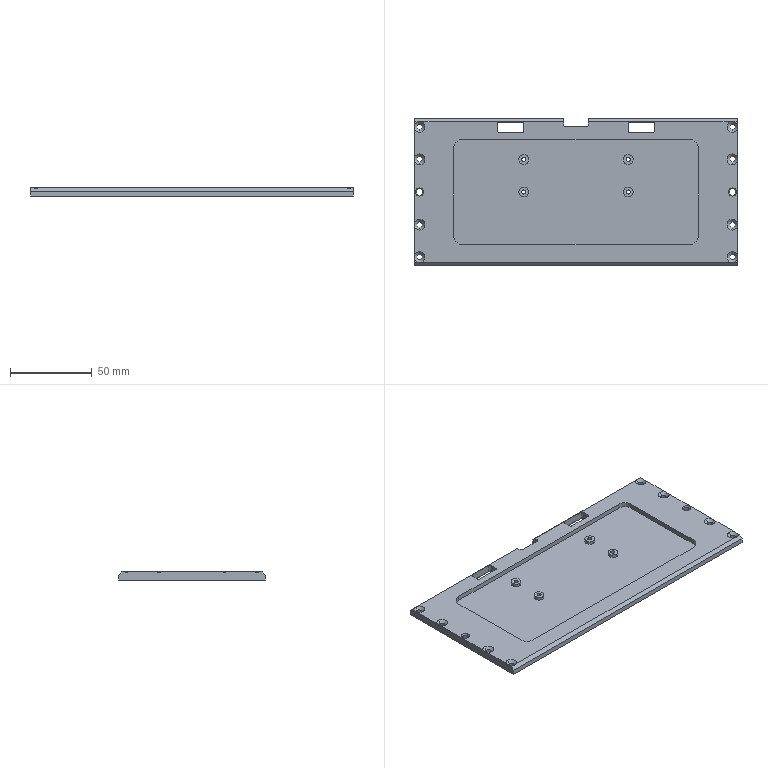NC program | NX | posted with a generic post | part box 198 x 90 x 5 mm
Lines 1 to 1736 of 7766:
N10 G17 G21 G94 G90
(DRILLING , TOOL : D6A45)
N12 T01 M6
N14 G54
N16 G17 G0 G90 X96. Y0. S5000 M3
N18 G43 Z30. H1
N20 G94 G81 G98 Z-2.5 F350. R3.
N22 X-96.
N24 G80
N26 G0 X-96. Y0. Z30.
(DRILLING_COPY_COPY , TOOL : D6A45)
N28 X96. Y-40.
N30 G81 Z-1. F350. R3.
N32 Y-20.
N34 Y20.
N36 Y40.
N38 X32. Y20.
N40 Y0.
N42 X-32.
N44 Y20.
N46 X-96. Y40.
N48 Y20.
N50 Y-20.
N52 Y-40.
N54 G80
N56 G0 X-96. Y-40. Z30.
N58 M5
(DRILLING_COPY_1_COPY , TOOL : 3.4ZT)
N60 T16 M6
N62 G54
N64 G17 G0 G90 X-96. Y-40. S2000 M3
N66 G43 Z30. H16
N68 G94 G83 G98 Z-6.521 F200. Q2. R3.
N70 Y-20.
N72 Y20.
N74 Y40.
N76 X96.
N78 Y20.
N80 Y-20.
N82 Y-40.
N84 G80
N86 G0 X96. Y-40. Z30.
N88 M5
(DRILLING_COPY_1_COPY_COPY , TOOL : 2.5ZT)
N90 T02 M6
N92 G54
N94 G17 G0 G90 X32. Y0. S2000 M3
N96 G43 Z30. H2
N98 G94 G83 G98 Z-6.251 F200. Q2. R3.
N100 Y20.
N102 X-32. Y0.
N104 Y20.
N106 G80
N108 G0 X-32. Y20. Z30.
N110 M5
(ZLEVEL_PROFILE_COPY_1_COPY , TOOL : D10)
N112 T15 M6
N114 G54
N116 G17 G0 G90 X104.1 Y-13.918 S9500 M3
N118 G43 Z30. H15
N120 Z1.5
N122 G94 G1 Y-45.554 Z-0.158 F1000.
N124 X103.766 Y-46.898 Z-0.231
N126 X103.084 Y-48.104 Z-0.303
N128 X102.104 Y-49.084 Z-0.376
N130 X100.898 Y-49.766 Z-0.448
N132 X99.554 Y-50.1 Z-0.521
N134 X99. Z-0.55
N136 X-99. F3000.
N138 G2 X-104.1 Y-45. R5.1
N140 G1 Y45.
N142 G2 X-99. Y50.1 R5.1
N144 G1 X-7.5
N146 G2 X-2.401 Y45.1 R5.1
N148 G1 X2.401
N150 G2 X7.5 Y50.1 R5.1
N152 G1 X99.
N154 G2 X104.1 Y45. R5.1
N156 G1 Y-45.
N158 G2 X99. Y-50.1 R5.1
N160 G1 X-89.1 Z-0.719
N162 X-94.05 Z-0.723
N164 X-99. Z-0.727
N166 X-99.5 Y-50.075 Z-0.728
N168 X-99.995 Y-50.002
N170 X-100.48 Y-49.88 Z-0.729
N172 X-100.952 Y-49.712
N174 X-101.404 Y-49.498 Z-0.73
N176 X-101.833 Y-49.24
N178 X-102.235 Y-48.942 Z-0.731
N180 X-102.606 Y-48.606
N182 X-102.942 Y-48.235 Z-0.732
N184 X-103.24 Y-47.833
N186 X-103.498 Y-47.404
N188 X-103.712 Y-46.952 Z-0.733
N190 X-103.88 Y-46.48
N192 X-104.002 Y-45.995 Z-0.734
N194 X-104.075 Y-45.5
N196 X-104.1 Y-45. Z-0.735
N198 X-104.103 Y-40. Z-0.739
N200 X-104.1 Y-35. Z-0.744
N202 Y35. Z-0.806
N204 X-104.103 Y40. Z-0.811
N206 X-104.1 Y45. Z-0.815
N208 X-104.075 Y45.5 Z-0.816
N210 X-104.002 Y45.995
N212 X-103.88 Y46.48 Z-0.817
N214 X-103.712 Y46.952
N216 X-103.498 Y47.404 Z-0.818
N218 X-103.24 Y47.833
N220 X-102.942 Y48.235
N222 X-102.606 Y48.606 Z-0.819
N224 X-102.235 Y48.942
N226 X-101.833 Y49.24 Z-0.82
N228 X-101.404 Y49.498
N230 X-100.952 Y49.712 Z-0.821
N232 X-100.48 Y49.88
N234 X-99.995 Y50.002 Z-0.822
N236 X-99.5 Y50.075
N238 X-99. Y50.1
N240 X-7.5 Z-0.905
N242 X-7.006 Y50.076
N244 X-6.517 Y50.004
N246 X-6.038 Y49.886 Z-0.906
N248 X-5.571 Y49.721
N250 X-5.123 Y49.512 Z-0.907
N252 X-4.698 Y49.261
N254 X-4.299 Y48.97 Z-0.908
N256 X-3.929 Y48.641
N258 X-3.594 Y48.279
N260 X-3.295 Y47.885 Z-0.909
N262 X-3.035 Y47.465
N264 X-2.817 Y47.021 Z-0.91
N266 X-2.644 Y46.558
N268 X-2.516 Y46.081 Z-0.911
N270 X-2.436 Y45.603
N272 X-2.401 Y45.1 Z-0.912
N274 X2.401 Z-0.916
N276 X2.436 Y45.603
N278 X2.516 Y46.081 Z-0.917
N280 X2.644 Y46.558
N282 X2.817 Y47.021 Z-0.918
N284 X3.035 Y47.465
N286 X3.295 Y47.885 Z-0.919
N288 X3.594 Y48.279
N290 X3.929 Y48.641
N292 X4.299 Y48.97 Z-0.92
N294 X4.698 Y49.261
N296 X5.123 Y49.512 Z-0.921
N298 X5.571 Y49.721
N300 X6.038 Y49.886 Z-0.922
N302 X6.517 Y50.004
N304 X7.006 Y50.076 Z-0.923
N306 X7.5 Y50.1
N308 X99. Z-1.005
N310 X99.5 Y50.075
N312 X99.995 Y50.002 Z-1.006
N314 X100.48 Y49.88
N316 X100.952 Y49.712 Z-1.007
N318 X101.404 Y49.498
N320 X101.833 Y49.24 Z-1.008
N322 X102.235 Y48.942
N324 X102.606 Y48.606 Z-1.009
N326 X102.942 Y48.235
N328 X103.24 Y47.833
N330 X103.498 Y47.404 Z-1.01
N332 X103.712 Y46.952
N334 X103.88 Y46.48 Z-1.011
N336 X104.002 Y45.995
N338 X104.075 Y45.5 Z-1.012
N340 X104.1 Y45.
N342 X104.105 Y40.5 Z-1.016
N344 X104.1 Y36. Z-1.02
N346 Y-36. Z-1.085
N348 X104.105 Y-40.5 Z-1.089
N350 X104.1 Y-45. Z-1.093
N352 X104.075 Y-45.5
N354 X104.002 Y-45.995 Z-1.094
N356 X103.88 Y-46.48
N358 X103.712 Y-46.952 Z-1.095
N360 X103.498 Y-47.404
N362 X103.24 Y-47.833 Z-1.096
N364 X102.942 Y-48.235
N366 X102.606 Y-48.606
N368 X102.235 Y-48.942 Z-1.097
N370 X101.833 Y-49.24
N372 X101.404 Y-49.498 Z-1.098
N374 X100.952 Y-49.712
N376 X100.48 Y-49.88 Z-1.099
N378 X99.995 Y-50.002
N380 X99.5 Y-50.075 Z-1.1
N382 X99. Y-50.1
N384 X-89.1 Z-1.269
N386 X-94.05 Z-1.273
N388 X-99. Z-1.277
N390 X-99.5 Y-50.075 Z-1.278
N392 X-99.995 Y-50.002
N394 X-100.48 Y-49.88 Z-1.279
N396 X-100.952 Y-49.712
N398 X-101.404 Y-49.498 Z-1.28
N400 X-101.833 Y-49.24
N402 X-102.235 Y-48.942 Z-1.281
N404 X-102.606 Y-48.606
N406 X-102.942 Y-48.235 Z-1.282
N408 X-103.24 Y-47.833
N410 X-103.498 Y-47.404
N412 X-103.712 Y-46.952 Z-1.283
N414 X-103.88 Y-46.48
N416 X-104.002 Y-45.995 Z-1.284
N418 X-104.075 Y-45.5
N420 X-104.1 Y-45. Z-1.285
N422 X-104.103 Y-40. Z-1.289
N424 X-104.1 Y-35. Z-1.294
N426 Y35. Z-1.356
N428 X-104.103 Y40. Z-1.361
N430 X-104.1 Y45. Z-1.365
N432 X-104.075 Y45.5 Z-1.366
N434 X-104.002 Y45.995
N436 X-103.88 Y46.48 Z-1.367
N438 X-103.712 Y46.952
N440 X-103.498 Y47.404 Z-1.368
N442 X-103.24 Y47.833
N444 X-102.942 Y48.235
N446 X-102.606 Y48.606 Z-1.369
N448 X-102.235 Y48.942
N450 X-101.833 Y49.24 Z-1.37
N452 X-101.404 Y49.498
N454 X-100.952 Y49.712 Z-1.371
N456 X-100.48 Y49.88
N458 X-99.995 Y50.002 Z-1.372
N460 X-99.5 Y50.075
N462 X-99. Y50.1
N464 X-7.5 Z-1.455
N466 X-7.006 Y50.076
N468 X-6.517 Y50.004
N470 X-6.038 Y49.886 Z-1.456
N472 X-5.571 Y49.721
N474 X-5.123 Y49.512 Z-1.457
N476 X-4.698 Y49.261
N478 X-4.299 Y48.97 Z-1.458
N480 X-3.929 Y48.641
N482 X-3.594 Y48.279
N484 X-3.295 Y47.885 Z-1.459
N486 X-3.035 Y47.465
N488 X-2.817 Y47.021 Z-1.46
N490 X-2.644 Y46.558
N492 X-2.516 Y46.081 Z-1.461
N494 X-2.436 Y45.603
N496 X-2.401 Y45.1 Z-1.462
N498 X2.401 Z-1.466
N500 X2.436 Y45.603
N502 X2.516 Y46.081 Z-1.467
N504 X2.644 Y46.558
N506 X2.817 Y47.021 Z-1.468
N508 X3.035 Y47.465
N510 X3.295 Y47.885 Z-1.469
N512 X3.594 Y48.279
N514 X3.929 Y48.641
N516 X4.299 Y48.97 Z-1.47
N518 X4.698 Y49.261
N520 X5.123 Y49.512 Z-1.471
N522 X5.571 Y49.721
N524 X6.038 Y49.886 Z-1.472
N526 X6.517 Y50.004
N528 X7.006 Y50.076 Z-1.473
N530 X7.5 Y50.1
N532 X99. Z-1.555
N534 X99.5 Y50.075
N536 X99.995 Y50.002 Z-1.556
N538 X100.48 Y49.88
N540 X100.952 Y49.712 Z-1.557
N542 X101.404 Y49.498
N544 X101.833 Y49.24 Z-1.558
N546 X102.235 Y48.942
N548 X102.606 Y48.606 Z-1.559
N550 X102.942 Y48.235
N552 X103.24 Y47.833
N554 X103.498 Y47.404 Z-1.56
N556 X103.712 Y46.952
N558 X103.88 Y46.48 Z-1.561
N560 X104.002 Y45.995
N562 X104.075 Y45.5 Z-1.562
N564 X104.1 Y45.
N566 X104.105 Y40.5 Z-1.566
N568 X104.1 Y36. Z-1.57
N570 Y-36. Z-1.635
N572 X104.105 Y-40.5 Z-1.639
N574 X104.1 Y-45. Z-1.643
N576 X104.075 Y-45.5
N578 X104.002 Y-45.995 Z-1.644
N580 X103.88 Y-46.48
N582 X103.712 Y-46.952 Z-1.645
N584 X103.498 Y-47.404
N586 X103.24 Y-47.833 Z-1.646
N588 X102.942 Y-48.235
N590 X102.606 Y-48.606
N592 X102.235 Y-48.942 Z-1.647
N594 X101.833 Y-49.24
N596 X101.404 Y-49.498 Z-1.648
N598 X100.952 Y-49.712
N600 X100.48 Y-49.88 Z-1.649
N602 X99.995 Y-50.002
N604 X99.5 Y-50.075 Z-1.65
N606 X99. Y-50.1
N608 X-89.1 Z-1.819
N610 X-94.05 Z-1.823
N612 X-99. Z-1.827
N614 X-99.5 Y-50.075 Z-1.828
N616 X-99.995 Y-50.002
N618 X-100.48 Y-49.88 Z-1.829
N620 X-100.952 Y-49.712
N622 X-101.404 Y-49.498 Z-1.83
N624 X-101.833 Y-49.24
N626 X-102.235 Y-48.942 Z-1.831
N628 X-102.606 Y-48.606
N630 X-102.942 Y-48.235 Z-1.832
N632 X-103.24 Y-47.833
N634 X-103.498 Y-47.404
N636 X-103.712 Y-46.952 Z-1.833
N638 X-103.88 Y-46.48
N640 X-104.002 Y-45.995 Z-1.834
N642 X-104.075 Y-45.5
N644 X-104.1 Y-45. Z-1.835
N646 X-104.103 Y-40. Z-1.839
N648 X-104.1 Y-35. Z-1.844
N650 Y35. Z-1.906
N652 X-104.103 Y40. Z-1.911
N654 X-104.1 Y45. Z-1.915
N656 X-104.075 Y45.5 Z-1.916
N658 X-104.002 Y45.995
N660 X-103.88 Y46.48 Z-1.917
N662 X-103.712 Y46.952
N664 X-103.498 Y47.404 Z-1.918
N666 X-103.24 Y47.833
N668 X-102.942 Y48.235
N670 X-102.606 Y48.606 Z-1.919
N672 X-102.235 Y48.942
N674 X-101.833 Y49.24 Z-1.92
N676 X-101.404 Y49.498
N678 X-100.952 Y49.712 Z-1.921
N680 X-100.48 Y49.88
N682 X-99.995 Y50.002 Z-1.922
N684 X-99.5 Y50.075
N686 X-99. Y50.1
N688 X-7.5 Z-2.005
N690 X-7.006 Y50.076
N692 X-6.517 Y50.004
N694 X-6.038 Y49.886 Z-2.006
N696 X-5.571 Y49.721
N698 X-5.123 Y49.512 Z-2.007
N700 X-4.698 Y49.261
N702 X-4.299 Y48.97 Z-2.008
N704 X-3.929 Y48.641
N706 X-3.594 Y48.279
N708 X-3.295 Y47.885 Z-2.009
N710 X-3.035 Y47.465
N712 X-2.817 Y47.021 Z-2.01
N714 X-2.644 Y46.558
N716 X-2.516 Y46.081 Z-2.011
N718 X-2.436 Y45.603
N720 X-2.401 Y45.1 Z-2.012
N722 X2.401 Z-2.016
N724 X2.436 Y45.603
N726 X2.516 Y46.081 Z-2.017
N728 X2.644 Y46.558
N730 X2.817 Y47.021 Z-2.018
N732 X3.035 Y47.465
N734 X3.295 Y47.885 Z-2.019
N736 X3.594 Y48.279
N738 X3.929 Y48.641
N740 X4.299 Y48.97 Z-2.02
N742 X4.698 Y49.261
N744 X5.123 Y49.512 Z-2.021
N746 X5.571 Y49.721
N748 X6.038 Y49.886 Z-2.022
N750 X6.517 Y50.004
N752 X7.006 Y50.076 Z-2.023
N754 X7.5 Y50.1
N756 X99. Z-2.105
N758 X99.5 Y50.075
N760 X99.995 Y50.002 Z-2.106
N762 X100.48 Y49.88
N764 X100.952 Y49.712 Z-2.107
N766 X101.404 Y49.498
N768 X101.833 Y49.24 Z-2.108
N770 X102.235 Y48.942
N772 X102.606 Y48.606 Z-2.109
N774 X102.942 Y48.235
N776 X103.24 Y47.833
N778 X103.498 Y47.404 Z-2.11
N780 X103.712 Y46.952
N782 X103.88 Y46.48 Z-2.111
N784 X104.002 Y45.995
N786 X104.075 Y45.5 Z-2.112
N788 X104.1 Y45.
N790 X104.105 Y40.5 Z-2.116
N792 X104.1 Y36. Z-2.12
N794 Y-36. Z-2.185
N796 X104.105 Y-40.5 Z-2.189
N798 X104.1 Y-45. Z-2.193
N800 X104.075 Y-45.5
N802 X104.002 Y-45.995 Z-2.194
N804 X103.88 Y-46.48
N806 X103.712 Y-46.952 Z-2.195
N808 X103.498 Y-47.404
N810 X103.24 Y-47.833 Z-2.196
N812 X102.942 Y-48.235
N814 X102.606 Y-48.606
N816 X102.235 Y-48.942 Z-2.197
N818 X101.833 Y-49.24
N820 X101.404 Y-49.498 Z-2.198
N822 X100.952 Y-49.712
N824 X100.48 Y-49.88 Z-2.199
N826 X99.995 Y-50.002
N828 X99.5 Y-50.075 Z-2.2
N830 X99. Y-50.1
N832 X-89.1 Z-2.369
N834 X-94.05 Z-2.373
N836 X-99. Z-2.377
N838 X-99.5 Y-50.075 Z-2.378
N840 X-99.995 Y-50.002
N842 X-100.48 Y-49.88 Z-2.379
N844 X-100.952 Y-49.712
N846 X-101.404 Y-49.498 Z-2.38
N848 X-101.833 Y-49.24
N850 X-102.235 Y-48.942 Z-2.381
N852 X-102.606 Y-48.606
N854 X-102.942 Y-48.235 Z-2.382
N856 X-103.24 Y-47.833
N858 X-103.498 Y-47.404
N860 X-103.712 Y-46.952 Z-2.383
N862 X-103.88 Y-46.48
N864 X-104.002 Y-45.995 Z-2.384
N866 X-104.075 Y-45.5
N868 X-104.1 Y-45. Z-2.385
N870 X-104.103 Y-40. Z-2.389
N872 X-104.1 Y-35. Z-2.394
N874 Y35. Z-2.456
N876 X-104.103 Y40. Z-2.461
N878 X-104.1 Y45. Z-2.465
N880 X-104.075 Y45.5 Z-2.466
N882 X-104.002 Y45.995
N884 X-103.88 Y46.48 Z-2.467
N886 X-103.712 Y46.952
N888 X-103.498 Y47.404 Z-2.468
N890 X-103.24 Y47.833
N892 X-102.942 Y48.235
N894 X-102.606 Y48.606 Z-2.469
N896 X-102.235 Y48.942
N898 X-101.833 Y49.24 Z-2.47
N900 X-101.404 Y49.498
N902 X-100.952 Y49.712 Z-2.471
N904 X-100.48 Y49.88
N906 X-99.995 Y50.002 Z-2.472
N908 X-99.5 Y50.075
N910 X-99. Y50.1
N912 X-7.5 Z-2.555
N914 X-7.006 Y50.076
N916 X-6.517 Y50.004
N918 X-6.038 Y49.886 Z-2.556
N920 X-5.571 Y49.721
N922 X-5.123 Y49.512 Z-2.557
N924 X-4.698 Y49.261
N926 X-4.299 Y48.97 Z-2.558
N928 X-3.929 Y48.641
N930 X-3.594 Y48.279
N932 X-3.295 Y47.885 Z-2.559
N934 X-3.035 Y47.465
N936 X-2.817 Y47.021 Z-2.56
N938 X-2.644 Y46.558
N940 X-2.516 Y46.081 Z-2.561
N942 X-2.436 Y45.603
N944 X-2.401 Y45.1 Z-2.562
N946 X2.401 Z-2.566
N948 X2.436 Y45.603
N950 X2.516 Y46.081 Z-2.567
N952 X2.644 Y46.558
N954 X2.817 Y47.021 Z-2.568
N956 X3.035 Y47.465
N958 X3.295 Y47.885 Z-2.569
N960 X3.594 Y48.279
N962 X3.929 Y48.641
N964 X4.299 Y48.97 Z-2.57
N966 X4.698 Y49.261
N968 X5.123 Y49.512 Z-2.571
N970 X5.571 Y49.721
N972 X6.038 Y49.886 Z-2.572
N974 X6.517 Y50.004
N976 X7.006 Y50.076 Z-2.573
N978 X7.5 Y50.1
N980 X99. Z-2.655
N982 X99.5 Y50.075
N984 X99.995 Y50.002 Z-2.656
N986 X100.48 Y49.88
N988 X100.952 Y49.712 Z-2.657
N990 X101.404 Y49.498
N992 X101.833 Y49.24 Z-2.658
N994 X102.235 Y48.942
N996 X102.606 Y48.606 Z-2.659
N998 X102.942 Y48.235
N1000 X103.24 Y47.833
N1002 X103.498 Y47.404 Z-2.66
N1004 X103.712 Y46.952
N1006 X103.88 Y46.48 Z-2.661
N1008 X104.002 Y45.995
N1010 X104.075 Y45.5 Z-2.662
N1012 X104.1 Y45.
N1014 X104.105 Y40.5 Z-2.666
N1016 X104.1 Y36. Z-2.67
N1018 Y-36. Z-2.735
N1020 X104.105 Y-40.5 Z-2.739
N1022 X104.1 Y-45. Z-2.743
N1024 X104.075 Y-45.5
N1026 X104.002 Y-45.995 Z-2.744
N1028 X103.88 Y-46.48
N1030 X103.712 Y-46.952 Z-2.745
N1032 X103.498 Y-47.404
N1034 X103.24 Y-47.833 Z-2.746
N1036 X102.942 Y-48.235
N1038 X102.606 Y-48.606
N1040 X102.235 Y-48.942 Z-2.747
N1042 X101.833 Y-49.24
N1044 X101.404 Y-49.498 Z-2.748
N1046 X100.952 Y-49.712
N1048 X100.48 Y-49.88 Z-2.749
N1050 X99.995 Y-50.002
N1052 X99.5 Y-50.075 Z-2.75
N1054 X99. Y-50.1
N1056 X-89.1 Z-2.919
N1058 X-94.05 Z-2.923
N1060 X-99. Z-2.927
N1062 X-99.5 Y-50.075 Z-2.928
N1064 X-99.995 Y-50.002
N1066 X-100.48 Y-49.88 Z-2.929
N1068 X-100.952 Y-49.712
N1070 X-101.404 Y-49.498 Z-2.93
N1072 X-101.833 Y-49.24
N1074 X-102.235 Y-48.942 Z-2.931
N1076 X-102.606 Y-48.606
N1078 X-102.942 Y-48.235 Z-2.932
N1080 X-103.24 Y-47.833
N1082 X-103.498 Y-47.404
N1084 X-103.712 Y-46.952 Z-2.933
N1086 X-103.88 Y-46.48
N1088 X-104.002 Y-45.995 Z-2.934
N1090 X-104.075 Y-45.5
N1092 X-104.1 Y-45. Z-2.935
N1094 X-104.103 Y-40. Z-2.939
N1096 X-104.1 Y-35. Z-2.944
N1098 Y35. Z-3.006
N1100 X-104.103 Y40. Z-3.011
N1102 X-104.1 Y45. Z-3.015
N1104 X-104.075 Y45.5 Z-3.016
N1106 X-104.002 Y45.995
N1108 X-103.88 Y46.48 Z-3.017
N1110 X-103.712 Y46.952
N1112 X-103.498 Y47.404 Z-3.018
N1114 X-103.24 Y47.833
N1116 X-102.942 Y48.235
N1118 X-102.606 Y48.606 Z-3.019
N1120 X-102.235 Y48.942
N1122 X-101.833 Y49.24 Z-3.02
N1124 X-101.404 Y49.498
N1126 X-100.952 Y49.712 Z-3.021
N1128 X-100.48 Y49.88
N1130 X-99.995 Y50.002 Z-3.022
N1132 X-99.5 Y50.075
N1134 X-99. Y50.1
N1136 X-7.5 Z-3.105
N1138 X-7.006 Y50.076
N1140 X-6.517 Y50.004
N1142 X-6.038 Y49.886 Z-3.106
N1144 X-5.571 Y49.721
N1146 X-5.123 Y49.512 Z-3.107
N1148 X-4.698 Y49.261
N1150 X-4.299 Y48.97 Z-3.108
N1152 X-3.929 Y48.641
N1154 X-3.594 Y48.279
N1156 X-3.295 Y47.885 Z-3.109
N1158 X-3.035 Y47.465
N1160 X-2.817 Y47.021 Z-3.11
N1162 X-2.644 Y46.558
N1164 X-2.516 Y46.081 Z-3.111
N1166 X-2.436 Y45.603
N1168 X-2.401 Y45.1 Z-3.112
N1170 X2.401 Z-3.116
N1172 X2.436 Y45.603
N1174 X2.516 Y46.081 Z-3.117
N1176 X2.644 Y46.558
N1178 X2.817 Y47.021 Z-3.118
N1180 X3.035 Y47.465
N1182 X3.295 Y47.885 Z-3.119
N1184 X3.594 Y48.279
N1186 X3.929 Y48.641
N1188 X4.299 Y48.97 Z-3.12
N1190 X4.698 Y49.261
N1192 X5.123 Y49.512 Z-3.121
N1194 X5.571 Y49.721
N1196 X6.038 Y49.886 Z-3.122
N1198 X6.517 Y50.004
N1200 X7.006 Y50.076 Z-3.123
N1202 X7.5 Y50.1
N1204 X99. Z-3.205
N1206 X99.5 Y50.075
N1208 X99.995 Y50.002 Z-3.206
N1210 X100.48 Y49.88
N1212 X100.952 Y49.712 Z-3.207
N1214 X101.404 Y49.498
N1216 X101.833 Y49.24 Z-3.208
N1218 X102.235 Y48.942
N1220 X102.606 Y48.606 Z-3.209
N1222 X102.942 Y48.235
N1224 X103.24 Y47.833
N1226 X103.498 Y47.404 Z-3.21
N1228 X103.712 Y46.952
N1230 X103.88 Y46.48 Z-3.211
N1232 X104.002 Y45.995
N1234 X104.075 Y45.5 Z-3.212
N1236 X104.1 Y45.
N1238 X104.105 Y40.5 Z-3.216
N1240 X104.1 Y36. Z-3.22
N1242 Y-36. Z-3.285
N1244 X104.105 Y-40.5 Z-3.289
N1246 X104.1 Y-45. Z-3.293
N1248 X104.075 Y-45.5
N1250 X104.002 Y-45.995 Z-3.294
N1252 X103.88 Y-46.48
N1254 X103.712 Y-46.952 Z-3.295
N1256 X103.498 Y-47.404
N1258 X103.24 Y-47.833 Z-3.296
N1260 X102.942 Y-48.235
N1262 X102.606 Y-48.606
N1264 X102.235 Y-48.942 Z-3.297
N1266 X101.833 Y-49.24
N1268 X101.404 Y-49.498 Z-3.298
N1270 X100.952 Y-49.712
N1272 X100.48 Y-49.88 Z-3.299
N1274 X99.995 Y-50.002
N1276 X99.5 Y-50.075 Z-3.3
N1278 X99. Y-50.1
N1280 X-89.1 Z-3.469
N1282 X-94.05 Z-3.473
N1284 X-99. Z-3.477
N1286 X-99.5 Y-50.075 Z-3.478
N1288 X-99.995 Y-50.002
N1290 X-100.48 Y-49.88 Z-3.479
N1292 X-100.952 Y-49.712
N1294 X-101.404 Y-49.498 Z-3.48
N1296 X-101.833 Y-49.24
N1298 X-102.235 Y-48.942 Z-3.481
N1300 X-102.606 Y-48.606
N1302 X-102.942 Y-48.235 Z-3.482
N1304 X-103.24 Y-47.833
N1306 X-103.498 Y-47.404
N1308 X-103.712 Y-46.952 Z-3.483
N1310 X-103.88 Y-46.48
N1312 X-104.002 Y-45.995 Z-3.484
N1314 X-104.075 Y-45.5
N1316 X-104.1 Y-45. Z-3.485
N1318 X-104.103 Y-40. Z-3.489
N1320 X-104.1 Y-35. Z-3.494
N1322 Y35. Z-3.556
N1324 X-104.103 Y40. Z-3.561
N1326 X-104.1 Y45. Z-3.565
N1328 X-104.075 Y45.5 Z-3.566
N1330 X-104.002 Y45.995
N1332 X-103.88 Y46.48 Z-3.567
N1334 X-103.712 Y46.952
N1336 X-103.498 Y47.404 Z-3.568
N1338 X-103.24 Y47.833
N1340 X-102.942 Y48.235
N1342 X-102.606 Y48.606 Z-3.569
N1344 X-102.235 Y48.942
N1346 X-101.833 Y49.24 Z-3.57
N1348 X-101.404 Y49.498
N1350 X-100.952 Y49.712 Z-3.571
N1352 X-100.48 Y49.88
N1354 X-99.995 Y50.002 Z-3.572
N1356 X-99.5 Y50.075
N1358 X-99. Y50.1
N1360 X-7.5 Z-3.655
N1362 X-7.006 Y50.076
N1364 X-6.517 Y50.004
N1366 X-6.038 Y49.886 Z-3.656
N1368 X-5.571 Y49.721
N1370 X-5.123 Y49.512 Z-3.657
N1372 X-4.698 Y49.261
N1374 X-4.299 Y48.97 Z-3.658
N1376 X-3.929 Y48.641
N1378 X-3.594 Y48.279
N1380 X-3.295 Y47.885 Z-3.659
N1382 X-3.035 Y47.465
N1384 X-2.817 Y47.021 Z-3.66
N1386 X-2.644 Y46.558
N1388 X-2.516 Y46.081 Z-3.661
N1390 X-2.436 Y45.603
N1392 X-2.401 Y45.1 Z-3.662
N1394 X2.401 Z-3.666
N1396 X2.436 Y45.603
N1398 X2.516 Y46.081 Z-3.667
N1400 X2.644 Y46.558
N1402 X2.817 Y47.021 Z-3.668
N1404 X3.035 Y47.465
N1406 X3.295 Y47.885 Z-3.669
N1408 X3.594 Y48.279
N1410 X3.929 Y48.641
N1412 X4.299 Y48.97 Z-3.67
N1414 X4.698 Y49.261
N1416 X5.123 Y49.512 Z-3.671
N1418 X5.571 Y49.721
N1420 X6.038 Y49.886 Z-3.672
N1422 X6.517 Y50.004
N1424 X7.006 Y50.076 Z-3.673
N1426 X7.5 Y50.1
N1428 X99. Z-3.755
N1430 X99.5 Y50.075
N1432 X99.995 Y50.002 Z-3.756
N1434 X100.48 Y49.88
N1436 X100.952 Y49.712 Z-3.757
N1438 X101.404 Y49.498
N1440 X101.833 Y49.24 Z-3.758
N1442 X102.235 Y48.942
N1444 X102.606 Y48.606 Z-3.759
N1446 X102.942 Y48.235
N1448 X103.24 Y47.833
N1450 X103.498 Y47.404 Z-3.76
N1452 X103.712 Y46.952
N1454 X103.88 Y46.48 Z-3.761
N1456 X104.002 Y45.995
N1458 X104.075 Y45.5 Z-3.762
N1460 X104.1 Y45.
N1462 X104.105 Y40.5 Z-3.766
N1464 X104.1 Y36. Z-3.77
N1466 Y-36. Z-3.835
N1468 X104.105 Y-40.5 Z-3.839
N1470 X104.1 Y-45. Z-3.843
N1472 X104.075 Y-45.5
N1474 X104.002 Y-45.995 Z-3.844
N1476 X103.88 Y-46.48
N1478 X103.712 Y-46.952 Z-3.845
N1480 X103.498 Y-47.404
N1482 X103.24 Y-47.833 Z-3.846
N1484 X102.942 Y-48.235
N1486 X102.606 Y-48.606
N1488 X102.235 Y-48.942 Z-3.847
N1490 X101.833 Y-49.24
N1492 X101.404 Y-49.498 Z-3.848
N1494 X100.952 Y-49.712
N1496 X100.48 Y-49.88 Z-3.849
N1498 X99.995 Y-50.002
N1500 X99.5 Y-50.075 Z-3.85
N1502 X99. Y-50.1
N1504 X-89.1 Z-4.019
N1506 X-94.05 Z-4.023
N1508 X-99. Z-4.027
N1510 X-99.5 Y-50.075 Z-4.028
N1512 X-99.995 Y-50.002
N1514 X-100.48 Y-49.88 Z-4.029
N1516 X-100.952 Y-49.712
N1518 X-101.404 Y-49.498 Z-4.03
N1520 X-101.833 Y-49.24
N1522 X-102.235 Y-48.942 Z-4.031
N1524 X-102.606 Y-48.606
N1526 X-102.942 Y-48.235 Z-4.032
N1528 X-103.24 Y-47.833
N1530 X-103.498 Y-47.404
N1532 X-103.712 Y-46.952 Z-4.033
N1534 X-103.88 Y-46.48
N1536 X-104.002 Y-45.995 Z-4.034
N1538 X-104.075 Y-45.5
N1540 X-104.1 Y-45. Z-4.035
N1542 X-104.103 Y-40. Z-4.039
N1544 X-104.1 Y-35. Z-4.044
N1546 Y35. Z-4.106
N1548 X-104.103 Y40. Z-4.111
N1550 X-104.1 Y45. Z-4.115
N1552 X-104.075 Y45.5 Z-4.116
N1554 X-104.002 Y45.995
N1556 X-103.88 Y46.48 Z-4.117
N1558 X-103.712 Y46.952
N1560 X-103.498 Y47.404 Z-4.118
N1562 X-103.24 Y47.833
N1564 X-102.942 Y48.235
N1566 X-102.606 Y48.606 Z-4.119
N1568 X-102.235 Y48.942
N1570 X-101.833 Y49.24 Z-4.12
N1572 X-101.404 Y49.498
N1574 X-100.952 Y49.712 Z-4.121
N1576 X-100.48 Y49.88
N1578 X-99.995 Y50.002 Z-4.122
N1580 X-99.5 Y50.075
N1582 X-99. Y50.1
N1584 X-7.5 Z-4.205
N1586 X-7.006 Y50.076
N1588 X-6.517 Y50.004
N1590 X-6.038 Y49.886 Z-4.206
N1592 X-5.571 Y49.721
N1594 X-5.123 Y49.512 Z-4.207
N1596 X-4.698 Y49.261
N1598 X-4.299 Y48.97 Z-4.208
N1600 X-3.929 Y48.641
N1602 X-3.594 Y48.279
N1604 X-3.295 Y47.885 Z-4.209
N1606 X-3.035 Y47.465
N1608 X-2.817 Y47.021 Z-4.21
N1610 X-2.644 Y46.558
N1612 X-2.516 Y46.081 Z-4.211
N1614 X-2.436 Y45.603
N1616 X-2.401 Y45.1 Z-4.212
N1618 X2.401 Z-4.216
N1620 X2.436 Y45.603
N1622 X2.516 Y46.081 Z-4.217
N1624 X2.644 Y46.558
N1626 X2.817 Y47.021 Z-4.218
N1628 X3.035 Y47.465
N1630 X3.295 Y47.885 Z-4.219
N1632 X3.594 Y48.279
N1634 X3.929 Y48.641
N1636 X4.299 Y48.97 Z-4.22
N1638 X4.698 Y49.261
N1640 X5.123 Y49.512 Z-4.221
N1642 X5.571 Y49.721
N1644 X6.038 Y49.886 Z-4.222
N1646 X6.517 Y50.004
N1648 X7.006 Y50.076 Z-4.223
N1650 X7.5 Y50.1
N1652 X99. Z-4.305
N1654 X99.5 Y50.075
N1656 X99.995 Y50.002 Z-4.306
N1658 X100.48 Y49.88
N1660 X100.952 Y49.712 Z-4.307
N1662 X101.404 Y49.498
N1664 X101.833 Y49.24 Z-4.308
N1666 X102.235 Y48.942
N1668 X102.606 Y48.606 Z-4.309
N1670 X102.942 Y48.235
N1672 X103.24 Y47.833
N1674 X103.498 Y47.404 Z-4.31
N1676 X103.712 Y46.952
N1678 X103.88 Y46.48 Z-4.311
N1680 X104.002 Y45.995
N1682 X104.075 Y45.5 Z-4.312
N1684 X104.1 Y45.
N1686 X104.105 Y40.5 Z-4.316
N1688 X104.1 Y36. Z-4.32
N1690 Y-36. Z-4.385
N1692 X104.105 Y-40.5 Z-4.389
N1694 X104.1 Y-45. Z-4.393
N1696 X104.075 Y-45.5
N1698 X104.002 Y-45.995 Z-4.394
N1700 X103.88 Y-46.48
N1702 X103.712 Y-46.952 Z-4.395
N1704 X103.498 Y-47.404
N1706 X103.24 Y-47.833 Z-4.396
N1708 X102.942 Y-48.235
N1710 X102.606 Y-48.606
N1712 X102.235 Y-48.942 Z-4.397
N1714 X101.833 Y-49.24
N1716 X101.404 Y-49.498 Z-4.398
N1718 X100.952 Y-49.712
N1720 X100.48 Y-49.88 Z-4.399
N1722 X99.995 Y-50.002
N1724 X99.5 Y-50.075 Z-4.4
N1726 X99. Y-50.1
N1728 X-99.
N1730 G2 X-104.1 Y-45. R5.1
N1732 G1 Y45.
N1734 G2 X-99. Y50.1 R5.1
N1736 G1 X-7.5
N1738 G2 X-2.401 Y45.1 R5.1
N1740 G1 X2.401
N1742 G2 X7.5 Y50.1 R5.1
N1744 G1 X99.
N1746 G2 X104.1 Y45. R5.1
N1748 G1 Y-45.
N1750 G2 X99. Y-50.1 R5.1
N1752 G1 Z-2.9
N1754 G0 Z30.
(FLOOR_WALL , TOOL : D10)
N1756 X-0.422 Y-1.9
N1758 Z1.5
N1760 G1 X4.065 Z1.265 F1000.
N1762 X4. Y-0.951 Z1.215
N1764 X4.034 Y1.376 Z1.093
N1766 X3.86 Y1.636 Z1.077
N1768 X3.692 Y1.9 Z1.06
N1770 X-3.692 Z0.673
N1772 X-3.86 Y1.636 Z0.657
N1774 X-4.034 Y1.376 Z0.64
N1776 X-4. Y-0.951 Z0.518
N1778 X-4.065 Y-1.9 Z0.469
N1780 X4.065 Z0.043
N1782 X4. Y-0.951 Z-0.007
N1784 X4.034 Y1.376 Z-0.129
N1786 X3.86 Y1.636 Z-0.146
N1788 X3.692 Y1.9 Z-0.162
N1790 X-3.692 Z-0.549
N1792 X-3.86 Y1.636 Z-0.565
N1794 X-4.034 Y1.376 Z-0.582
N1796 X-4. Y-0.951 Z-0.704
N1798 X-4.065 Y-1.9 Z-0.754
N1800 X0. Z-0.967
N1802 X4.065 F3000.
N1804 G2 X4.034 Y1.376 R28.
N1806 X3.692 Y1.9 R33.6
N1808 G1 X-3.692
N1810 G2 X-4.034 Y1.376 R33.6
N1812 X-4.065 Y-1.9 R28.
N1814 G1 X0.
N1816 Y-6.4
N1818 X9.388
N1820 G2 X8.648 Y2.636 R23.5
N1822 X6.274 Y6.4 R29.1
N1824 G1 X-6.274
N1826 G2 X-8.648 Y2.636 R29.1
N1828 X-9.388 Y-6.4 R23.5
N1830 G1 X0.
N1832 Y-13.4
N1834 X22.372
N1836 X27.361 Y-13.738
N1838 G3 X36.639 Y-13.738 R14.5
N1840 X37.045 Y-15.4 R5.
N1842 G1 X26.955
N1844 G3 X27.361 Y-13.738 R5.
N1846 G1 X22.372 Y-13.4
N1848 G2 X16.153 Y4.596 R16.5
N1850 X10.909 Y13.4 R22.1
N1852 G1 X-10.909
N1854 G2 X-16.153 Y4.596 R22.1
N1856 X-22.372 Y-13.4 R16.5
N1858 G1 X-26.955 Y-15.4
N1860 X-37.045
N1862 G3 X-36.639 Y-13.738 R5.
N1864 X-27.361 Y-13.738 R14.5
N1866 X-26.955 Y-15.4 R5.
N1868 G1 X-22.372 Y-13.4
N1870 X0.
N1872 Y-20.4
N1874 X62.9
N1876 Y20.4
N1878 X47.095
N1880 G2 X38.875 Y6.556 R15.1
N1882 X40.605 Y-4.026 R9.5
N1884 G1 X51.021 Y-8.9
N1886 X51.4
N1888 Y-8.04
N1890 G2 X51.021 Y-8.9 R21.
N1892 G1 X46.945 Y-6.993
N1894 G2 X41.628 Y-13.4 R16.5
N1896 G1 X55.9
N1898 Y13.4
N1900 X53.091
N1902 G2 X47.847 Y4.596 R22.1
N1904 X46.945 Y-6.993 R16.5
N1906 G1 X40.605 Y-4.026
N1908 G2 X25.125 Y6.556 R-9.5
N1910 G1 X26.138 Y5.59
N1912 G2 X37.59 Y5.862 R8.1
N1914 X26.138 Y5.59 R-8.1
N1916 G1 X25.125 Y6.556
N1918 G2 X16.905 Y20.4 R15.1
N1920 G1 X-16.905
N1922 G2 X-25.125 Y6.556 R15.1
N1924 X-38.875 Y6.556 R-9.5
N1926 G1 X-37.862 Y5.59
N1928 G2 X-26.41 Y5.862 R8.1
N1930 X-37.862 Y5.59 R-8.1
N1932 G1 X-38.875 Y6.556
N1934 G2 X-47.095 Y20.4 R15.1
N1936 G1 X-62.9
N1938 Y-20.4
N1940 X-51.021
N1942 Y-8.9
N1944 G2 X-51.4 Y-8.04 R21.
N1946 G1 Y-8.9
N1948 X-51.021
N1950 Y-13.4
N1952 X-41.628
N1954 G2 X-47.847 Y4.596 R16.5
N1956 X-53.091 Y13.4 R22.1
N1958 G1 X-55.9
N1960 Y-13.4
N1962 X-51.021
N1964 Y-20.4
N1966 X0.
N1968 Y-27.4
N1970 X69.
N1972 G3 X69.9 Y-26.5 R0.9
N1974 G1 Y26.5
N1976 G3 X69. Y27.4 R0.9
N1978 G1 X35.294
N1980 G2 X28.706 Y27.4 R-8.1
N1982 G1 X-28.706
N1984 G2 X-35.294 Y27.4 R-8.1
N1986 G1 X-69.
N1988 G3 X-69.9 Y26.5 R0.9
N1990 G1 Y-26.5
N1992 G3 X-69. Y-27.4 R0.9
N1994 G1 X0.
N1996 Z0.533
N1998 G0 X-0.422 Y-1.9
N2000 G1 X4.065 Z0.298 F1000.
N2002 X4. Y-0.951 Z0.248
N2004 X4.034 Y1.376 Z0.126
N2006 X3.86 Y1.636 Z0.11
N2008 X3.692 Y1.9 Z0.094
N2010 X-3.692 Z-0.293
N2012 X-3.86 Y1.636 Z-0.31
N2014 X-4.034 Y1.376 Z-0.326
N2016 X-4. Y-0.951 Z-0.448
N2018 X-4.065 Y-1.9 Z-0.498
N2020 X4.065 Z-0.924
N2022 X4. Y-0.951 Z-0.974
N2024 X4.034 Y1.376 Z-1.096
N2026 X3.86 Y1.636 Z-1.112
N2028 X3.692 Y1.9 Z-1.129
N2030 X-3.692 Z-1.516
N2032 X-3.86 Y1.636 Z-1.532
N2034 X-4.034 Y1.376 Z-1.548
N2036 X-4. Y-0.951 Z-1.67
N2038 X-4.065 Y-1.9 Z-1.72
N2040 X0. Z-1.933
N2042 X4.065 F3000.
N2044 G2 X4.034 Y1.376 R28.
N2046 X3.692 Y1.9 R33.6
N2048 G1 X-3.692
N2050 G2 X-4.034 Y1.376 R33.6
N2052 X-4.065 Y-1.9 R28.
N2054 G1 X0.
N2056 Y-6.4
N2058 X9.388
N2060 G2 X8.648 Y2.636 R23.5
N2062 X6.274 Y6.4 R29.1
N2064 G1 X-6.274
N2066 G2 X-8.648 Y2.636 R29.1
N2068 X-9.388 Y-6.4 R23.5
N2070 G1 X0.
N2072 Y-13.4
N2074 X22.372
N2076 X27.361 Y-13.738
N2078 G3 X36.639 Y-13.738 R14.5
N2080 X37.045 Y-15.4 R5.
N2082 G1 X26.955
N2084 G3 X27.361 Y-13.738 R5.
N2086 G1 X22.372 Y-13.4
N2088 G2 X16.153 Y4.596 R16.5
N2090 X10.909 Y13.4 R22.1
N2092 G1 X-10.909
N2094 G2 X-16.153 Y4.596 R22.1
N2096 X-22.372 Y-13.4 R16.5
N2098 G1 X-26.955 Y-15.4
N2100 X-37.045
N2102 G3 X-36.639 Y-13.738 R5.
N2104 X-27.361 Y-13.738 R14.5
N2106 X-26.955 Y-15.4 R5.
N2108 G1 X-22.372 Y-13.4
N2110 X0.
N2112 Y-20.4
N2114 X62.9
N2116 Y20.4
N2118 X47.095
N2120 G2 X38.875 Y6.556 R15.1
N2122 X40.605 Y-4.026 R9.5
N2124 G1 X51.021 Y-8.9
N2126 X51.4
N2128 Y-8.04
N2130 G2 X51.021 Y-8.9 R21.
N2132 G1 X46.945 Y-6.993
N2134 G2 X41.628 Y-13.4 R16.5
N2136 G1 X55.9
N2138 Y13.4
N2140 X53.091
N2142 G2 X47.847 Y4.596 R22.1
N2144 X46.945 Y-6.993 R16.5
N2146 G1 X40.605 Y-4.026
N2148 G2 X25.125 Y6.556 R-9.5
N2150 G1 X26.138 Y5.59
N2152 G2 X37.59 Y5.862 R8.1
N2154 X26.138 Y5.59 R-8.1
N2156 G1 X25.125 Y6.556
N2158 G2 X16.905 Y20.4 R15.1
N2160 G1 X-16.905
N2162 G2 X-25.125 Y6.556 R15.1
N2164 X-38.875 Y6.556 R-9.5
N2166 G1 X-37.862 Y5.59
N2168 G2 X-26.41 Y5.862 R8.1
N2170 X-37.862 Y5.59 R-8.1
N2172 G1 X-38.875 Y6.556
N2174 G2 X-47.095 Y20.4 R15.1
N2176 G1 X-62.9
N2178 Y-20.4
N2180 X-51.021
N2182 Y-8.9
N2184 G2 X-51.4 Y-8.04 R21.
N2186 G1 Y-8.9
N2188 X-51.021
N2190 Y-13.4
N2192 X-41.628
N2194 G2 X-47.847 Y4.596 R16.5
N2196 X-53.091 Y13.4 R22.1
N2198 G1 X-55.9
N2200 Y-13.4
N2202 X-51.021
N2204 Y-20.4
N2206 X0.
N2208 Y-27.4
N2210 X69.
N2212 G3 X69.9 Y-26.5 R0.9
N2214 G1 Y26.5
N2216 G3 X69. Y27.4 R0.9
N2218 G1 X35.294
N2220 G2 X28.706 Y27.4 R-8.1
N2222 G1 X-28.706
N2224 G2 X-35.294 Y27.4 R-8.1
N2226 G1 X-69.
N2228 G3 X-69.9 Y26.5 R0.9
N2230 G1 Y-26.5
N2232 G3 X-69. Y-27.4 R0.9
N2234 G1 X0.
N2236 Z-0.433
N2238 G0 X-0.422 Y-1.9
N2240 G1 X4.065 Z-0.668 F1000.
N2242 X4. Y-0.951 Z-0.718
N2244 X4.034 Y1.376 Z-0.84
N2246 X3.86 Y1.636 Z-0.857
N2248 X3.692 Y1.9 Z-0.873
N2250 X-3.692 Z-1.26
N2252 X-3.86 Y1.636 Z-1.276
N2254 X-4.034 Y1.376 Z-1.293
N2256 X-4. Y-0.951 Z-1.415
N2258 X-4.065 Y-1.9 Z-1.465
N2260 X4.065 Z-1.891
N2262 X4. Y-0.951 Z-1.941
N2264 X4.034 Y1.376 Z-2.063
N2266 X3.86 Y1.636 Z-2.079
N2268 X3.692 Y1.9 Z-2.095
N2270 X-3.692 Z-2.482
N2272 X-3.86 Y1.636 Z-2.499
N2274 X-4.034 Y1.376 Z-2.515
N2276 X-4. Y-0.951 Z-2.637
N2278 X-4.065 Y-1.9 Z-2.687
N2280 X0. Z-2.9
N2282 X4.065 F3000.
N2284 G2 X4.034 Y1.376 R28.
N2286 X3.692 Y1.9 R33.6
N2288 G1 X-3.692
N2290 G2 X-4.034 Y1.376 R33.6
N2292 X-4.065 Y-1.9 R28.
N2294 G1 X0.
N2296 Y-6.4
N2298 X9.388
N2300 G2 X8.648 Y2.636 R23.5
N2302 X6.274 Y6.4 R29.1
N2304 G1 X-6.274
N2306 G2 X-8.648 Y2.636 R29.1
N2308 X-9.388 Y-6.4 R23.5
N2310 G1 X0.
N2312 Y-13.4
N2314 X22.372
N2316 X27.361 Y-13.738
N2318 G3 X36.639 Y-13.738 R14.5
N2320 X37.045 Y-15.4 R5.
N2322 G1 X26.955
N2324 G3 X27.361 Y-13.738 R5.
N2326 G1 X22.372 Y-13.4
N2328 G2 X16.153 Y4.596 R16.5
N2330 X10.909 Y13.4 R22.1
N2332 G1 X-10.909
N2334 G2 X-16.153 Y4.596 R22.1
N2336 X-22.372 Y-13.4 R16.5
N2338 G1 X-26.955 Y-15.4
N2340 X-37.045
N2342 G3 X-36.639 Y-13.738 R5.
N2344 X-27.361 Y-13.738 R14.5
N2346 X-26.955 Y-15.4 R5.
N2348 G1 X-22.372 Y-13.4
N2350 X0.
N2352 Y-20.4
N2354 X62.9
N2356 Y20.4
N2358 X47.095
N2360 G2 X38.875 Y6.556 R15.1
N2362 X40.605 Y-4.026 R9.5
N2364 G1 X51.021 Y-8.9
N2366 X51.4
N2368 Y-8.04
N2370 G2 X51.021 Y-8.9 R21.
N2372 G1 X46.945 Y-6.993
N2374 G2 X41.628 Y-13.4 R16.5
N2376 G1 X55.9
N2378 Y13.4
N2380 X53.091
N2382 G2 X47.847 Y4.596 R22.1
N2384 X46.945 Y-6.993 R16.5
N2386 G1 X40.605 Y-4.026
N2388 G2 X25.125 Y6.556 R-9.5
N2390 G1 X26.138 Y5.59
N2392 G2 X37.59 Y5.862 R8.1
N2394 X26.138 Y5.59 R-8.1
N2396 G1 X25.125 Y6.556
N2398 G2 X16.905 Y20.4 R15.1
N2400 G1 X-16.905
N2402 G2 X-25.125 Y6.556 R15.1
N2404 X-38.875 Y6.556 R-9.5
N2406 G1 X-37.862 Y5.59
N2408 G2 X-26.41 Y5.862 R8.1
N2410 X-37.862 Y5.59 R-8.1
N2412 G1 X-38.875 Y6.556
N2414 G2 X-47.095 Y20.4 R15.1
N2416 G1 X-62.9
N2418 Y-20.4
N2420 X-51.021
N2422 Y-8.9
N2424 G2 X-51.4 Y-8.04 R21.
N2426 G1 Y-8.9
N2428 X-51.021
N2430 Y-13.4
N2432 X-41.628
N2434 G2 X-47.847 Y4.596 R16.5
N2436 X-53.091 Y13.4 R22.1
N2438 G1 X-55.9
N2440 Y-13.4
N2442 X-51.021
N2444 Y-20.4
N2446 X0.
N2448 Y-27.4
N2450 X69.
N2452 G3 X69.9 Y-26.5 R0.9
N2454 G1 Y26.5
N2456 G3 X69. Y27.4 R0.9
N2458 G1 X35.294
N2460 G2 X28.706 Y27.4 R-8.1
N2462 G1 X-28.706
N2464 G2 X-35.294 Y27.4 R-8.1
N2466 G1 X-69.
N2468 G3 X-69.9 Y26.5 R0.9
N2470 G1 Y-26.5
N2472 G3 X-69. Y-27.4 R0.9
N2474 G1 X0.
N2476 Z-1.4
N2478 G0 Z30.
(FLOOR_WALL_COPY_1 , TOOL : D10)
N2480 X-27.508 Y-7.799
N2482 Z0.1
N2484 G1 Z-0.9 F1000.
N2486 X-31.234 Y-3.357
N2488 G3 X-32. Y-3. R1.
N2490 G2 X-35. Y0. R3. F3000.
N2492 X-32. Y-3. R-3.
N2494 G3 X-32.766 Y-3.357 R1.
N2496 G1 X-36.493 Y-7.798
N2498 Z0.1
N2500 G0 Z30.
N2502 X-38.328 Y26.4
N2504 Z0.1
N2506 G1 Z-0.9 F1000.
N2508 X-32.766 Y23.357
N2510 G3 X-32. Y23. R1.
N2512 G2 X-29. Y20. R3. F3000.
N2514 X-32. Y23. R-3.
N2516 G3 X-31.234 Y23.357 R1.
N2518 G1 X-25.672 Y26.4
N2520 Z0.1
N2522 G0 Z30.
N2524 X25.672
N2526 Z0.1
N2528 G1 Z-0.9 F1000.
N2530 X31.234 Y23.357
N2532 G3 X32. Y23. R1.
N2534 G2 X35. Y20. R3. F3000.
N2536 X32. Y23. R-3.
N2538 G3 X32.766 Y23.357 R1.
N2540 G1 X38.328 Y26.4
N2542 Z0.1
N2544 G0 Z30.
N2546 X27.507 Y7.798
N2548 Z0.1
N2550 G1 Z-0.9 F1000.
N2552 X31.234 Y3.357
N2554 G3 X32. Y3. R1.
N2556 G2 X35. Y0. R3. F3000.
N2558 X32. Y3. R-3.
N2560 G3 X32.766 Y3.357 R1.
N2562 G1 X36.493 Y7.798
N2564 Z0.1
N2566 G0 Z30.
N2568 M5
(FLOOR_WALL_COPY , TOOL : D6)
N2570 T12 M6
N2572 G54
N2574 G17 G0 G90 X-33.192 Y27.405 S9500 M3
N2576 G43 Z30. H12
N2578 Z0.
N2580 G94 G1 Z-1. F1000.
N2582 X-32.555 Y26.3
N2584 G3 X-32.035 Y26. R0.6
N2586 G1 X-31.965 F1500.
N2588 G2 X-27.357 Y23.8 R6.
N2590 G1 X-36.643
N2592 G3 X-37.783 Y21.6 R6.
N2594 G1 X-26.217
N2596 G2 X-26.03 Y19.4 R6.
N2598 G1 X-37.97
N2600 G2 X-38.49 Y19.7 R0.6
N2602 G1 X-39.393 Y21.264
N2604 Z0.
N2606 G0 Z30.
N2608 X-33.192 Y7.405
N2610 Z0.
N2612 G1 Z-1. F1000.
N2614 X-32.555 Y6.3
N2616 G3 X-32.035 Y6. R0.6
N2618 G1 X-31.965 F1500.
N2620 G2 X-27.357 Y3.8 R6.
N2622 G1 X-36.643
N2624 G3 X-37.783 Y1.6 R6.
N2626 G1 X-26.217
N2628 G2 X-26.03 Y-0.6 R6.
N2630 G1 X-37.97
N2632 G2 X-38.49 Y-0.3 R0.6
N2634 G1 X-39.393 Y1.264
N2636 Z0.
N2638 G0 Z30.
N2640 X-68.554 Y28.899
N2642 Z-2.
N2644 G1 Z-3. F1000.
N2646 G3 X-69.073 Y29.199 R0.6
N2648 G1 X69.073 F1500.
N2650 G2 X71.7 Y26.5 R2.7
N2652 G1 Y26.279
N2654 X32.513
N2656 G2 X37.33 Y23.359 R6.3
N2658 G1 X71.7
N2660 Y20.439
N2662 X38.285
N2664 G2 X37.791 Y17.519 R6.3
N2666 G1 X71.7
N2668 Y14.599
N2670 X35.244
N2672 Z-2.
N2674 G0 Z30.
N2676 X-31.994 Y26.579
N2678 Z-2.
N2680 G1 Z-3. F1000.
N2682 G2 X-32.513 Y26.279 R0.6
N2684 G1 X-71.7 F1500.
N2686 Y23.359
N2688 X-37.33
N2690 G3 X-38.285 Y20.439 R6.3
N2692 G1 X-71.7
N2694 Y17.519
N2696 X-37.791
N2698 G3 X-35.244 Y14.599 R6.3
N2700 G1 X-71.7
N2702 Z-2.
N2704 G0 Z30.
N2706 X32.006 Y26.579
N2708 Z-2.
N2710 G1 Z-3. F1000.
N2712 G2 X31.487 Y26.279 R0.6
N2714 G1 X-31.487 F1500.
N2716 G2 X-26.67 Y23.359 R6.3
N2718 G1 X26.67
N2720 G3 X25.715 Y20.439 R6.3
N2722 G1 X-25.715
N2724 G2 X-26.209 Y17.519 R6.3
N2726 G1 X26.209
N2728 G3 X28.756 Y14.599 R6.3
N2730 G1 X-28.756
N2732 Z-2.
N2734 G0 Z30.
N2736 X-71.4 Y12.199
N2738 Z-2.
N2740 G1 Z-3. F1000.
N2742 G3 X-71.7 Y11.679 R0.6
N2744 G1 X71.7 F1500.
N2746 Y8.759
N2748 X-71.7
N2750 Y5.839
N2752 X-34.365
N2754 G3 X-37.583 Y2.919 R6.3
N2756 G1 X-71.7
N2758 Y0.
N2760 X-38.3
N2762 G3 X-37.582 Y-2.92 R6.3
N2764 G1 X-71.7
N2766 Y-5.84
N2768 X-34.362
N2770 G3 X-34.956 Y-5.924 R0.6
N2772 G1 Z-2.
N2774 G0 Z30.
N2776 X-30.004 Y6.313
N2778 Z-2.
N2780 G1 Z-3. F1000.
N2782 G3 X-29.635 Y5.839 R0.6
N2784 G1 X29.635 F1500.
N2786 G3 X26.417 Y2.919 R6.3
N2788 G1 X-26.417
N2790 G2 X-25.7 Y0. R6.3
N2792 G1 X25.7
N2794 G3 X26.418 Y-2.92 R6.3
N2796 G1 X-26.418
N2798 G2 X-29.638 Y-5.84 R6.3
N2800 G1 X29.638
N2802 G3 X29.044 Y-5.924 R0.6
N2804 G1 Z-2.
N2806 G0 Z30.
N2808 X33.996 Y6.313
N2810 Z-2.
N2812 G1 Z-3. F1000.
N2814 G3 X34.365 Y5.839 R0.6
N2816 G1 X71.7 F1500.
N2818 Y2.919
N2820 X37.583
N2822 G2 X38.3 Y0. R6.3
N2824 G1 X71.7
N2826 Y-2.92
N2828 X37.582
N2830 G2 X34.362 Y-5.84 R6.3
N2832 G1 X71.7
N2834 Y-8.76
N2836 X-71.7
N2838 Y-11.68
N2840 X71.7
N2842 Y-14.6
N2844 X-71.7
N2846 Y-17.52
N2848 X71.7
N2850 Y-20.44
N2852 X-71.7
N2854 Y-23.36
N2856 X71.7
N2858 Y-26.28
N2860 X-71.7
N2862 Y-26.5
N2864 G3 X-69.009 Y-29.2 R2.7
N2866 G1 X69.009
N2868 G3 X69.528 Y-28.9 R0.6
N2870 G1 Z-2.
N2872 G0 Z30.
N2874 X33.321 Y-7.687
N2876 Z-2.
N2878 G1 Z-3. F1000.
N2880 X32.52 Y-6.3
N2882 G3 X32. Y-6. R0.6
N2884 G2 X26. Y0. R6. F1500.
N2886 X32. Y-6. R-6.
N2888 G3 X31.48 Y-6.3 R0.6
N2890 G1 X30.679 Y-7.687
N2892 Z-2.
N2894 G0 Z30.
N2896 Y27.687
N2898 Z-2.
N2900 G1 Z-3. F1000.
N2902 X31.48 Y26.3
N2904 G3 X32. Y26. R0.6
N2906 G2 X38. Y20. R6. F1500.
N2908 X32. Y26. R-6.
N2910 G3 X32.52 Y26.3 R0.6
N2912 G1 X33.321 Y27.687
N2914 Z-2.
N2916 G0 Z30.
N2918 X-33.321
N2920 Z-2.
N2922 G1 Z-3. F1000.
N2924 X-32.52 Y26.3
N2926 G3 X-32. Y26. R0.6
N2928 G2 X-26. Y20. R6. F1500.
N2930 X-32. Y26. R-6.
N2932 G3 X-31.48 Y26.3 R0.6
N2934 G1 X-30.679 Y27.687
N2936 Z-2.
N2938 G0 Z30.
N2940 X-33.321 Y7.687
N2942 Z-2.
N2944 G1 Z-3. F1000.
N2946 X-32.52 Y6.3
N2948 G3 X-32. Y6. R0.6
N2950 G2 X-26. Y0. R6. F1500.
N2952 X-32. Y6. R-6.
N2954 G3 X-31.48 Y6.3 R0.6
N2956 G1 X-30.679 Y7.687
N2958 Z-2.
N2960 G0 Z30.
N2962 X1.386 Y27.7
N2964 Z-2.
N2966 G1 Z-3. F1000.
N2968 X0.52 Y29.2
N2970 G3 X0. Y29.5 R0.6
N2972 G1 X-69. F1500.
N2974 G3 X-72. Y26.5 R3.
N2976 G1 Y-26.5
N2978 G3 X-69. Y-29.5 R3.
N2980 G1 X69.
N2982 G3 X72. Y-26.5 R3.
N2984 G1 Y26.5
N2986 G3 X69. Y29.5 R3.
N2988 G1 X0.
N2990 G3 X-0.52 Y29.2 R0.6
N2992 G1 X-1.212 Y28.
N2994 Z-2.
N2996 G0 Z30.
N2998 X30.807 Y7.405
N3000 Z0.
N3002 G1 Z-1. F1000.
N3004 X31.445 Y6.3
N3006 G3 X31.965 Y6. R0.6
N3008 G1 X32.034 F1500.
N3010 G2 X36.643 Y3.8 R6.
N3012 G1 X27.356
N3014 G3 X26.217 Y1.6 R6.
N3016 G1 X37.783
N3018 G2 X37.97 Y-0.6 R6.
N3020 G1 X26.03
N3022 G2 X25.51 Y-0.3 R0.6
N3024 G1 X24.607 Y1.264
N3026 Z0.
N3028 G0 Z30.
N3030 X30.807 Y27.405
N3032 Z0.
N3034 G1 Z-1. F1000.
N3036 X31.445 Y26.3
N3038 G3 X31.965 Y26. R0.6
N3040 G1 X32.034 F1500.
N3042 G2 X36.643 Y23.8 R6.
N3044 G1 X27.356
N3046 G3 X26.217 Y21.6 R6.
N3048 G1 X37.783
N3050 G2 X37.97 Y19.4 R6.
N3052 G1 X26.03
N3054 G2 X25.51 Y19.7 R0.6
N3056 G1 X24.607 Y21.264
N3058 Z0.
N3060 G0 Z30.
N3062 M5
(ZLEVEL_PROFILE_COPY_1_COPY_COPY , TOOL : D4)
N3064 T11 M6
N3066 G54
N3068 G17 G0 G90 X-38.861 Y38.5 S9500 M3
N3070 G43 Z30. H11
N3072 Z1.5
N3074 G94 G1 X-33.9 Z1.24 F1000.
N3076 Y40.7 Z1.125
N3078 X-46.1 Z0.485
N3080 Y38.5 Z0.37
N3082 X-33.9 Z-0.269
N3084 Y40.7 Z-0.385
N3086 X-46.1 F2000.
N3088 Y38.5
N3090 X-33.9
N3092 Y40.7
N3094 X-46.1 Z-0.548
N3096 Y38.5 Z-0.577
N3098 X-33.9 Z-0.74
N3100 Y40.7 Z-0.769
N3102 X-45.859 Z-0.929
N3104 X-46.1 Y40.697 Z-0.932
N3106 Y38.5 Z-0.962
N3108 X-34.141 Z-1.121
N3110 X-33.9 Y38.503 Z-1.125
N3112 Y40.7 Z-1.154
N3114 X-45.859 Z-1.314
N3116 X-46.1 Y40.697 Z-1.317
N3118 Y38.5 Z-1.346
N3120 X-34.141 Z-1.506
N3122 X-33.9 Y38.503 Z-1.509
N3124 Y40.7 Z-1.538
N3126 X-45.859 Z-1.698
N3128 X-46.1 Y40.697 Z-1.701
N3130 Y38.5 Z-1.731
N3132 X-34.141 Z-1.89
N3134 X-33.9 Y38.503 Z-1.894
N3136 Y40.7 Z-1.923
N3138 X-45.859 Z-2.083
N3140 X-46.1 Y40.697 Z-2.086
N3142 Y38.5 Z-2.115
N3144 X-34.141 Z-2.275
N3146 X-33.9 Y38.503 Z-2.278
N3148 Y40.7 Z-2.308
N3150 X-45.859 Z-2.467
N3152 X-46.1 Y40.697 Z-2.471
N3154 Y38.5 Z-2.5
N3156 X-34.141 Z-2.66
N3158 X-33.9 Y38.503 Z-2.663
N3160 Y40.7 Z-2.692
N3162 X-45.859 Z-2.852
N3164 X-46.1 Y40.697 Z-2.855
N3166 Y38.5 Z-2.885
N3168 X-34.141 Z-3.044
N3170 X-33.9 Y38.503 Z-3.048
N3172 Y40.7 Z-3.077
N3174 X-45.859 Z-3.237
N3176 X-46.1 Y40.697 Z-3.24
N3178 Y38.5 Z-3.269
N3180 X-34.141 Z-3.429
N3182 X-33.9 Y38.503 Z-3.432
N3184 Y40.7 Z-3.462
N3186 X-45.859 Z-3.621
N3188 X-46.1 Y40.697 Z-3.625
N3190 Y38.5 Z-3.654
N3192 X-34.141 Z-3.814
N3194 X-33.9 Y38.503 Z-3.817
N3196 Y40.7 Z-3.846
N3198 X-45.859 Z-4.006
N3200 X-46.1 Y40.697 Z-4.009
N3202 Y38.5 Z-4.038
N3204 X-34.141 Z-4.198
N3206 X-33.9 Y38.503 Z-4.201
N3208 Y40.7 Z-4.231
N3210 X-45.859 Z-4.39
N3212 X-46.1 Y40.697 Z-4.394
N3214 Y38.5 Z-4.423
N3216 X-34.141 Z-4.583
N3218 X-33.9 Y38.503 Z-4.586
N3220 Y40.7 Z-4.615
N3222 X-45.859 Z-4.775
N3224 X-46.1 Y40.697 Z-4.778
N3226 Y38.5 Z-4.808
N3228 X-34.141 Z-4.967
N3230 X-33.9 Y38.503 Z-4.971
N3232 Y40.7 Z-5.
N3234 X-46.1
N3236 Y38.5
N3238 X-33.9
N3240 Y40.7
N3242 Z-3.5
N3244 G0 Z30.
N3246 X41.139 Y38.5
N3248 Z1.5
N3250 G1 X46.1 Z1.24 F1000.
N3252 Y40.7 Z1.125
N3254 X33.9 Z0.485
N3256 Y38.5 Z0.37
N3258 X46.1 Z-0.269
N3260 Y40.7 Z-0.385
N3262 X33.9 F2000.
N3264 Y38.5
N3266 X46.1
N3268 Y40.7
N3270 X33.9 Z-0.548
N3272 Y38.5 Z-0.577
N3274 X46.1 Z-0.74
N3276 Y40.7 Z-0.769
N3278 X34.141 Z-0.929
N3280 X33.9 Y40.697 Z-0.932
N3282 Y38.5 Z-0.962
N3284 X45.859 Z-1.121
N3286 X46.1 Y38.503 Z-1.125
N3288 Y40.7 Z-1.154
N3290 X34.141 Z-1.314
N3292 X33.9 Y40.697 Z-1.317
N3294 Y38.5 Z-1.346
N3296 X45.859 Z-1.506
N3298 X46.1 Y38.503 Z-1.509
N3300 Y40.7 Z-1.538
N3302 X34.141 Z-1.698
N3304 X33.9 Y40.697 Z-1.701
N3306 Y38.5 Z-1.731
N3308 X45.859 Z-1.89
N3310 X46.1 Y38.503 Z-1.894
N3312 Y40.7 Z-1.923
N3314 X34.141 Z-2.083
N3316 X33.9 Y40.697 Z-2.086
N3318 Y38.5 Z-2.115
N3320 X45.859 Z-2.275
N3322 X46.1 Y38.503 Z-2.278
N3324 Y40.7 Z-2.308
N3326 X34.141 Z-2.467
N3328 X33.9 Y40.697 Z-2.471
N3330 Y38.5 Z-2.5
N3332 X45.859 Z-2.66
N3334 X46.1 Y38.503 Z-2.663
N3336 Y40.7 Z-2.692
N3338 X34.141 Z-2.852
N3340 X33.9 Y40.697 Z-2.855
N3342 Y38.5 Z-2.885
N3344 X45.859 Z-3.044
N3346 X46.1 Y38.503 Z-3.048
N3348 Y40.7 Z-3.077
N3350 X34.141 Z-3.237
N3352 X33.9 Y40.697 Z-3.24
N3354 Y38.5 Z-3.269
N3356 X45.859 Z-3.429
N3358 X46.1 Y38.503 Z-3.432
N3360 Y40.7 Z-3.462
N3362 X34.141 Z-3.621
N3364 X33.9 Y40.697 Z-3.625
N3366 Y38.5 Z-3.654
N3368 X45.859 Z-3.814
N3370 X46.1 Y38.503 Z-3.817
N3372 Y40.7 Z-3.846
N3374 X34.141 Z-4.006
N3376 X33.9 Y40.697 Z-4.009
N3378 Y38.5 Z-4.038
N3380 X45.859 Z-4.198
N3382 X46.1 Y38.503 Z-4.201
N3384 Y40.7 Z-4.231
N3386 X34.141 Z-4.39
N3388 X33.9 Y40.697 Z-4.394
N3390 Y38.5 Z-4.423
N3392 X45.859 Z-4.583
N3394 X46.1 Y38.503 Z-4.586
N3396 Y40.7 Z-4.615
N3398 X34.141 Z-4.775
N3400 X33.9 Y40.697 Z-4.778
N3402 Y38.5 Z-4.808
N3404 X45.859 Z-4.967
N3406 X46.1 Y38.503 Z-4.971
N3408 Y40.7 Z-5.
N3410 X33.9
N3412 Y38.5
N3414 X46.1
N3416 Y40.7
N3418 Z-3.5
N3420 G0 Z30.
N3422 M5